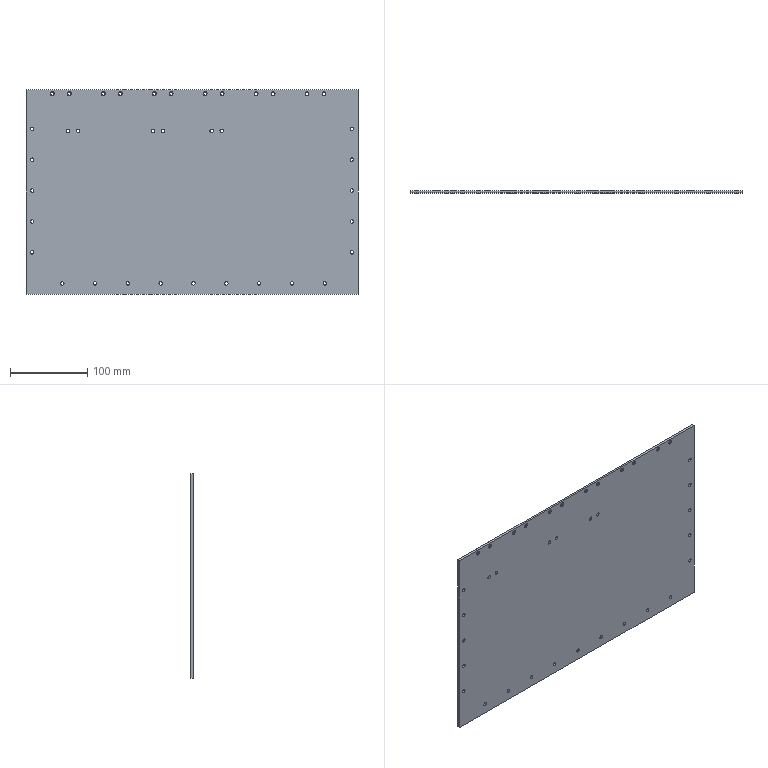Part | STEP file | Chassis left side panel | 1 solid | 67 faces | box 430 x 3 x 264.7 mm | volume 339377 mm3 | cylinder 37 | cone 24 | plane 6 | commonest cylinder face diameters 4.5 x25 4.3 x12